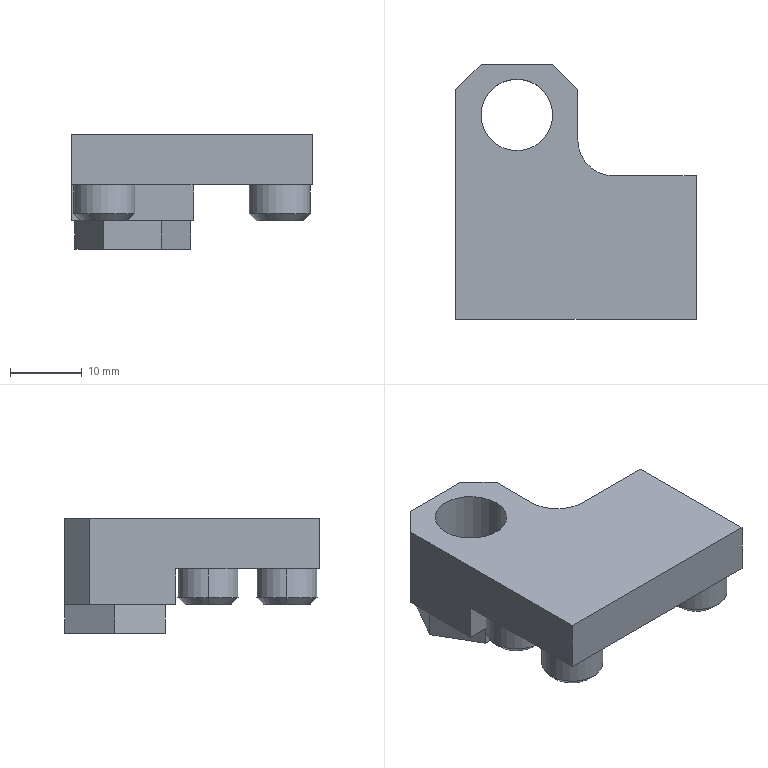Part | NX | 1 solid | 69 faces | box 33.5 x 35.5 x 16 mm | volume 8014 mm3 | plane 50 | cylinder 11 | cone 8 | commonest cylinder face diameters 8.5 x8 10 x3